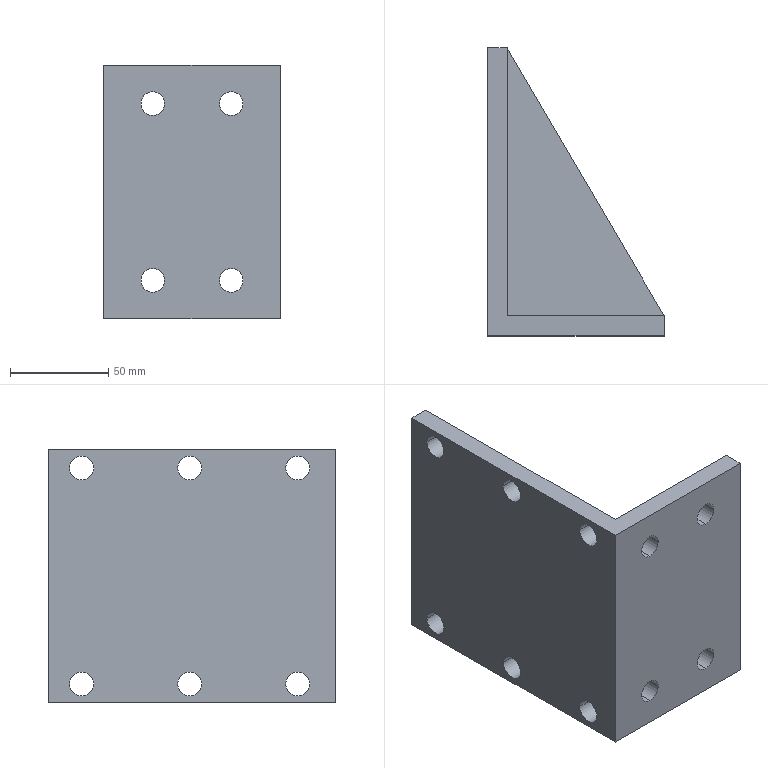Part | SolidWorks | features BaseBody 1, HoleWzd 1 | 1 solid | 33 faces | box 90 x 146.4 x 128.8 mm | volume 334625 mm3 | cylinder 20 | plane 13 | commonest cylinder face diameters 12.2 x12 12 x8
STEP:
#1=CARTESIAN_POINT('',(147.,10.6,14.));
#2=VERTEX_POINT('',#1);
#3=CARTESIAN_POINT('',(147.,10.6,26.));
#4=VERTEX_POINT('',#3);
#5=CARTESIAN_POINT('',(147.,10.6,20.));
#6=DIRECTION('',(0.,1.,0.));
#7=DIRECTION('',(-1.,0.,0.));
#8=AXIS2_PLACEMENT_3D('',#5,#6,#7);
#9=CIRCLE('',#8,6.);
#10=EDGE_CURVE('',#2,#4,#9,.T.);
#11=ORIENTED_EDGE('',*,*,#10,.T.);
#12=CARTESIAN_POINT('',(147.,0.6,26.));
#13=VERTEX_POINT('',#12);
#14=CARTESIAN_POINT('',(147.,0.6,26.));
#15=DIRECTION('',(0.,-1.,0.));
#16=VECTOR('',#15,1000.);
#17=LINE('',#14,#16);
#18=EDGE_CURVE('',#4,#13,#17,.T.);
#19=ORIENTED_EDGE('',*,*,#18,.T.);
#20=CARTESIAN_POINT('',(147.,0.6,14.));
#21=VERTEX_POINT('',#20);
#22=CARTESIAN_POINT('',(147.,0.6,20.));
#23=DIRECTION('',(0.,-1.,0.));
#24=DIRECTION('',(0.,0.,-1.));
#25=AXIS2_PLACEMENT_3D('',#22,#23,#24);
#26=CIRCLE('',#25,6.);
#27=EDGE_CURVE('',#13,#21,#26,.T.);
#28=ORIENTED_EDGE('',*,*,#27,.T.);
#29=CARTESIAN_POINT('',(147.,0.6,14.));
#30=DIRECTION('',(0.,-1.,0.));
#31=VECTOR('',#30,1000.);
#32=LINE('',#29,#31);
#33=EDGE_CURVE('',#2,#21,#32,.T.);
#34=ORIENTED_EDGE('',*,*,#33,.F.);
#35=EDGE_LOOP('',(#11,#19,#28,#34));
#36=FACE_OUTER_BOUND('',#35,.T.);
#37=CARTESIAN_POINT('',(147.,0.6,20.));
#38=DIRECTION('',(0.,-1.,0.));
#39=DIRECTION('',(0.,0.,-1.));
#40=AXIS2_PLACEMENT_3D('',#37,#38,#39);
#41=CYLINDRICAL_SURFACE('',#40,6.);
#42=ADVANCED_FACE('',(#36),#41,.F.);
#43=CARTESIAN_POINT('',(187.,10.6,14.));
#44=VERTEX_POINT('',#43);
#45=CARTESIAN_POINT('',(187.,10.6,26.));
#46=VERTEX_POINT('',#45);
#47=CARTESIAN_POINT('',(187.,10.6,20.));
#48=DIRECTION('',(0.,1.,0.));
#49=DIRECTION('',(-1.,0.,0.));
#50=AXIS2_PLACEMENT_3D('',#47,#48,#49);
#51=CIRCLE('',#50,6.);
#52=EDGE_CURVE('',#44,#46,#51,.T.);
#53=ORIENTED_EDGE('',*,*,#52,.T.);
#54=CARTESIAN_POINT('',(187.,0.6,26.));
#55=VERTEX_POINT('',#54);
#56=CARTESIAN_POINT('',(187.,0.6,26.));
#57=DIRECTION('',(0.,-1.,0.));
#58=VECTOR('',#57,1000.);
#59=LINE('',#56,#58);
#60=EDGE_CURVE('',#46,#55,#59,.T.);
#61=ORIENTED_EDGE('',*,*,#60,.T.);
#62=CARTESIAN_POINT('',(187.,0.6,14.));
#63=VERTEX_POINT('',#62);
#64=CARTESIAN_POINT('',(187.,0.6,20.));
#65=DIRECTION('',(0.,-1.,0.));
#66=DIRECTION('',(0.,0.,-1.));
#67=AXIS2_PLACEMENT_3D('',#64,#65,#66);
#68=CIRCLE('',#67,6.);
#69=EDGE_CURVE('',#55,#63,#68,.T.);
#70=ORIENTED_EDGE('',*,*,#69,.T.);
#71=CARTESIAN_POINT('',(187.,0.6,14.));
#72=DIRECTION('',(0.,-1.,0.));
#73=VECTOR('',#72,1000.);
#74=LINE('',#71,#73);
#75=EDGE_CURVE('',#44,#63,#74,.T.);
#76=ORIENTED_EDGE('',*,*,#75,.F.);
#77=EDGE_LOOP('',(#53,#61,#70,#76));
#78=FACE_OUTER_BOUND('',#77,.T.);
#79=CARTESIAN_POINT('',(187.,0.6,20.));
#80=DIRECTION('',(0.,-1.,0.));
#81=DIRECTION('',(0.,0.,-1.));
#82=AXIS2_PLACEMENT_3D('',#79,#80,#81);
#83=CYLINDRICAL_SURFACE('',#82,6.);
#84=ADVANCED_FACE('',(#78),#83,.F.);
#85=CARTESIAN_POINT('',(187.,10.6,104.));
#86=VERTEX_POINT('',#85);
#87=CARTESIAN_POINT('',(187.,10.6,116.));
#88=VERTEX_POINT('',#87);
#89=CARTESIAN_POINT('',(187.,10.6,110.));
#90=DIRECTION('',(0.,1.,0.));
#91=DIRECTION('',(-1.,0.,0.));
#92=AXIS2_PLACEMENT_3D('',#89,#90,#91);
#93=CIRCLE('',#92,6.);
#94=EDGE_CURVE('',#86,#88,#93,.T.);
#95=ORIENTED_EDGE('',*,*,#94,.T.);
#96=CARTESIAN_POINT('',(187.,0.6,116.));
#97=VERTEX_POINT('',#96);
#98=CARTESIAN_POINT('',(187.,0.6,116.));
#99=DIRECTION('',(0.,-1.,0.));
#100=VECTOR('',#99,1000.);
#101=LINE('',#98,#100);
#102=EDGE_CURVE('',#88,#97,#101,.T.);
#103=ORIENTED_EDGE('',*,*,#102,.T.);
#104=CARTESIAN_POINT('',(187.,0.6,104.));
#105=VERTEX_POINT('',#104);
#106=CARTESIAN_POINT('',(187.,0.6,110.));
#107=DIRECTION('',(0.,-1.,0.));
#108=DIRECTION('',(0.,0.,-1.));
#109=AXIS2_PLACEMENT_3D('',#106,#107,#108);
#110=CIRCLE('',#109,6.);
#111=EDGE_CURVE('',#97,#105,#110,.T.);
#112=ORIENTED_EDGE('',*,*,#111,.T.);
#113=CARTESIAN_POINT('',(187.,0.6,104.));
#114=DIRECTION('',(0.,-1.,0.));
#115=VECTOR('',#114,1000.);
#116=LINE('',#113,#115);
#117=EDGE_CURVE('',#86,#105,#116,.T.);
#118=ORIENTED_EDGE('',*,*,#117,.F.);
#119=EDGE_LOOP('',(#95,#103,#112,#118));
#120=FACE_OUTER_BOUND('',#119,.T.);
#121=CARTESIAN_POINT('',(187.,0.6,110.));
#122=DIRECTION('',(0.,-1.,0.));
#123=DIRECTION('',(0.,0.,-1.));
#124=AXIS2_PLACEMENT_3D('',#121,#122,#123);
#125=CYLINDRICAL_SURFACE('',#124,6.);
#126=ADVANCED_FACE('',(#120),#125,.F.);
#127=CARTESIAN_POINT('',(147.,10.6,104.));
#128=VERTEX_POINT('',#127);
#129=CARTESIAN_POINT('',(147.,10.6,116.));
#130=VERTEX_POINT('',#129);
#131=CARTESIAN_POINT('',(147.,10.6,110.));
#132=DIRECTION('',(0.,1.,0.));
#133=DIRECTION('',(-1.,0.,0.));
#134=AXIS2_PLACEMENT_3D('',#131,#132,#133);
#135=CIRCLE('',#134,6.);
#136=EDGE_CURVE('',#128,#130,#135,.T.);
#137=ORIENTED_EDGE('',*,*,#136,.T.);
#138=CARTESIAN_POINT('',(147.,0.6,116.));
#139=VERTEX_POINT('',#138);
#140=CARTESIAN_POINT('',(147.,0.6,116.));
#141=DIRECTION('',(0.,-1.,0.));
#142=VECTOR('',#141,1000.);
#143=LINE('',#140,#142);
#144=EDGE_CURVE('',#130,#139,#143,.T.);
#145=ORIENTED_EDGE('',*,*,#144,.T.);
#146=CARTESIAN_POINT('',(147.,0.6,104.));
#147=VERTEX_POINT('',#146);
#148=CARTESIAN_POINT('',(147.,0.6,110.));
#149=DIRECTION('',(0.,-1.,0.));
#150=DIRECTION('',(0.,0.,-1.));
#151=AXIS2_PLACEMENT_3D('',#148,#149,#150);
#152=CIRCLE('',#151,6.);
#153=EDGE_CURVE('',#139,#147,#152,.T.);
#154=ORIENTED_EDGE('',*,*,#153,.T.);
#155=CARTESIAN_POINT('',(147.,0.6,104.));
#156=DIRECTION('',(0.,-1.,0.));
#157=VECTOR('',#156,1000.);
#158=LINE('',#155,#157);
#159=EDGE_CURVE('',#128,#147,#158,.T.);
#160=ORIENTED_EDGE('',*,*,#159,.F.);
#161=EDGE_LOOP('',(#137,#145,#154,#160));
#162=FACE_OUTER_BOUND('',#161,.T.);
#163=CARTESIAN_POINT('',(147.,0.6,110.));
#164=DIRECTION('',(0.,-1.,0.));
#165=DIRECTION('',(0.,0.,-1.));
#166=AXIS2_PLACEMENT_3D('',#163,#164,#165);
#167=CYLINDRICAL_SURFACE('',#166,6.);
#168=ADVANCED_FACE('',(#162),#167,.F.);
#169=CARTESIAN_POINT('',(132.,68.9,10.));
#170=VERTEX_POINT('',#169);
#171=CARTESIAN_POINT('',(132.,81.1,10.));
#172=VERTEX_POINT('',#171);
#173=CARTESIAN_POINT('',(132.,75.,10.));
#174=DIRECTION('',(1.,0.,0.));
#175=DIRECTION('',(0.,1.,0.));
#176=AXIS2_PLACEMENT_3D('',#173,#174,#175);
#177=CIRCLE('',#176,6.1);
#178=EDGE_CURVE('',#170,#172,#177,.T.);
#179=ORIENTED_EDGE('',*,*,#178,.T.);
#180=CARTESIAN_POINT('',(122.,81.1,10.));
#181=VERTEX_POINT('',#180);
#182=CARTESIAN_POINT('',(132.,81.1,10.));
#183=DIRECTION('',(-1.,0.,0.));
#184=VECTOR('',#183,1000.);
#185=LINE('',#182,#184);
#186=EDGE_CURVE('',#172,#181,#185,.T.);
#187=ORIENTED_EDGE('',*,*,#186,.T.);
#188=CARTESIAN_POINT('',(122.,68.9,10.));
#189=VERTEX_POINT('',#188);
#190=CARTESIAN_POINT('',(122.,75.,10.));
#191=DIRECTION('',(1.,0.,0.));
#192=DIRECTION('',(0.,1.,0.));
#193=AXIS2_PLACEMENT_3D('',#190,#191,#192);
#194=CIRCLE('',#193,6.1);
#195=EDGE_CURVE('',#189,#181,#194,.T.);
#196=ORIENTED_EDGE('',*,*,#195,.F.);
#197=CARTESIAN_POINT('',(132.,68.9,10.));
#198=DIRECTION('',(-1.,0.,0.));
#199=VECTOR('',#198,1000.);
#200=LINE('',#197,#199);
#201=EDGE_CURVE('',#170,#189,#200,.T.);
#202=ORIENTED_EDGE('',*,*,#201,.F.);
#203=EDGE_LOOP('',(#179,#187,#196,#202));
#204=FACE_OUTER_BOUND('',#203,.T.);
#205=CARTESIAN_POINT('',(132.,75.,10.));
#206=DIRECTION('',(-1.,0.,0.));
#207=DIRECTION('',(0.,-1.,0.));
#208=AXIS2_PLACEMENT_3D('',#205,#206,#207);
#209=CYLINDRICAL_SURFACE('',#208,6.1);
#210=ADVANCED_FACE('',(#204),#209,.F.);
#211=CARTESIAN_POINT('',(132.,123.9,10.));
#212=VERTEX_POINT('',#211);
#213=CARTESIAN_POINT('',(132.,136.1,10.));
#214=VERTEX_POINT('',#213);
#215=CARTESIAN_POINT('',(132.,130.,10.));
#216=DIRECTION('',(1.,0.,0.));
#217=DIRECTION('',(0.,1.,0.));
#218=AXIS2_PLACEMENT_3D('',#215,#216,#217);
#219=CIRCLE('',#218,6.1);
#220=EDGE_CURVE('',#212,#214,#219,.T.);
#221=ORIENTED_EDGE('',*,*,#220,.T.);
#222=CARTESIAN_POINT('',(122.,136.1,10.));
#223=VERTEX_POINT('',#222);
#224=CARTESIAN_POINT('',(132.,136.1,10.));
#225=DIRECTION('',(-1.,0.,0.));
#226=VECTOR('',#225,1000.);
#227=LINE('',#224,#226);
#228=EDGE_CURVE('',#214,#223,#227,.T.);
#229=ORIENTED_EDGE('',*,*,#228,.T.);
#230=CARTESIAN_POINT('',(122.,123.9,10.));
#231=VERTEX_POINT('',#230);
#232=CARTESIAN_POINT('',(122.,130.,10.));
#233=DIRECTION('',(1.,0.,0.));
#234=DIRECTION('',(0.,1.,0.));
#235=AXIS2_PLACEMENT_3D('',#232,#233,#234);
#236=CIRCLE('',#235,6.1);
#237=EDGE_CURVE('',#231,#223,#236,.T.);
#238=ORIENTED_EDGE('',*,*,#237,.F.);
#239=CARTESIAN_POINT('',(132.,123.9,10.));
#240=DIRECTION('',(-1.,0.,0.));
#241=VECTOR('',#240,1000.);
#242=LINE('',#239,#241);
#243=EDGE_CURVE('',#212,#231,#242,.T.);
#244=ORIENTED_EDGE('',*,*,#243,.F.);
#245=EDGE_LOOP('',(#221,#229,#238,#244));
#246=FACE_OUTER_BOUND('',#245,.T.);
#247=CARTESIAN_POINT('',(132.,130.,10.));
#248=DIRECTION('',(-1.,0.,0.));
#249=DIRECTION('',(0.,-1.,0.));
#250=AXIS2_PLACEMENT_3D('',#247,#248,#249);
#251=CYLINDRICAL_SURFACE('',#250,6.1);
#252=ADVANCED_FACE('',(#246),#251,.F.);
#253=CARTESIAN_POINT('',(132.,123.9,120.));
#254=VERTEX_POINT('',#253);
#255=CARTESIAN_POINT('',(132.,136.1,120.));
#256=VERTEX_POINT('',#255);
#257=CARTESIAN_POINT('',(132.,130.,120.));
#258=DIRECTION('',(1.,0.,0.));
#259=DIRECTION('',(0.,1.,0.));
#260=AXIS2_PLACEMENT_3D('',#257,#258,#259);
#261=CIRCLE('',#260,6.1);
#262=EDGE_CURVE('',#254,#256,#261,.T.);
#263=ORIENTED_EDGE('',*,*,#262,.T.);
#264=CARTESIAN_POINT('',(122.,136.1,120.));
#265=VERTEX_POINT('',#264);
#266=CARTESIAN_POINT('',(132.,136.1,120.));
#267=DIRECTION('',(-1.,0.,0.));
#268=VECTOR('',#267,1000.);
#269=LINE('',#266,#268);
#270=EDGE_CURVE('',#256,#265,#269,.T.);
#271=ORIENTED_EDGE('',*,*,#270,.T.);
#272=CARTESIAN_POINT('',(122.,123.9,120.));
#273=VERTEX_POINT('',#272);
#274=CARTESIAN_POINT('',(122.,130.,120.));
#275=DIRECTION('',(1.,0.,0.));
#276=DIRECTION('',(0.,1.,0.));
#277=AXIS2_PLACEMENT_3D('',#274,#275,#276);
#278=CIRCLE('',#277,6.1);
#279=EDGE_CURVE('',#273,#265,#278,.T.);
#280=ORIENTED_EDGE('',*,*,#279,.F.);
#281=CARTESIAN_POINT('',(132.,123.9,120.));
#282=DIRECTION('',(-1.,0.,0.));
#283=VECTOR('',#282,1000.);
#284=LINE('',#281,#283);
#285=EDGE_CURVE('',#254,#273,#284,.T.);
#286=ORIENTED_EDGE('',*,*,#285,.F.);
#287=EDGE_LOOP('',(#263,#271,#280,#286));
#288=FACE_OUTER_BOUND('',#287,.T.);
#289=CARTESIAN_POINT('',(132.,130.,120.));
#290=DIRECTION('',(-1.,0.,0.));
#291=DIRECTION('',(0.,-1.,0.));
#292=AXIS2_PLACEMENT_3D('',#289,#290,#291);
#293=CYLINDRICAL_SURFACE('',#292,6.1);
#294=ADVANCED_FACE('',(#288),#293,.F.);
#295=CARTESIAN_POINT('',(132.,68.9,120.));
#296=VERTEX_POINT('',#295);
#297=CARTESIAN_POINT('',(132.,81.1,120.));
#298=VERTEX_POINT('',#297);
#299=CARTESIAN_POINT('',(132.,75.,120.));
#300=DIRECTION('',(1.,0.,0.));
#301=DIRECTION('',(0.,1.,0.));
#302=AXIS2_PLACEMENT_3D('',#299,#300,#301);
#303=CIRCLE('',#302,6.1);
#304=EDGE_CURVE('',#296,#298,#303,.T.);
#305=ORIENTED_EDGE('',*,*,#304,.T.);
#306=CARTESIAN_POINT('',(122.,81.1,120.));
#307=VERTEX_POINT('',#306);
#308=CARTESIAN_POINT('',(132.,81.1,120.));
#309=DIRECTION('',(-1.,0.,0.));
#310=VECTOR('',#309,1000.);
#311=LINE('',#308,#310);
#312=EDGE_CURVE('',#298,#307,#311,.T.);
#313=ORIENTED_EDGE('',*,*,#312,.T.);
#314=CARTESIAN_POINT('',(122.,68.9,120.));
#315=VERTEX_POINT('',#314);
#316=CARTESIAN_POINT('',(122.,75.,120.));
#317=DIRECTION('',(1.,0.,0.));
#318=DIRECTION('',(0.,1.,0.));
#319=AXIS2_PLACEMENT_3D('',#316,#317,#318);
#320=CIRCLE('',#319,6.1);
#321=EDGE_CURVE('',#315,#307,#320,.T.);
#322=ORIENTED_EDGE('',*,*,#321,.F.);
#323=CARTESIAN_POINT('',(132.,68.9,120.));
#324=DIRECTION('',(-1.,0.,0.));
#325=VECTOR('',#324,1000.);
#326=LINE('',#323,#325);
#327=EDGE_CURVE('',#296,#315,#326,.T.);
#328=ORIENTED_EDGE('',*,*,#327,.F.);
#329=EDGE_LOOP('',(#305,#313,#322,#328));
#330=FACE_OUTER_BOUND('',#329,.T.);
#331=CARTESIAN_POINT('',(132.,75.,120.));
#332=DIRECTION('',(-1.,0.,0.));
#333=DIRECTION('',(0.,-1.,0.));
#334=AXIS2_PLACEMENT_3D('',#331,#332,#333);
#335=CYLINDRICAL_SURFACE('',#334,6.1);
#336=ADVANCED_FACE('',(#330),#335,.F.);
#337=CARTESIAN_POINT('',(132.,13.9,120.));
#338=VERTEX_POINT('',#337);
#339=CARTESIAN_POINT('',(132.,26.1,120.));
#340=VERTEX_POINT('',#339);
#341=CARTESIAN_POINT('',(132.,20.,120.));
#342=DIRECTION('',(1.,0.,0.));
#343=DIRECTION('',(0.,1.,0.));
#344=AXIS2_PLACEMENT_3D('',#341,#342,#343);
#345=CIRCLE('',#344,6.1);
#346=EDGE_CURVE('',#338,#340,#345,.T.);
#347=ORIENTED_EDGE('',*,*,#346,.T.);
#348=CARTESIAN_POINT('',(122.,26.1,120.));
#349=VERTEX_POINT('',#348);
#350=CARTESIAN_POINT('',(132.,26.1,120.));
#351=DIRECTION('',(-1.,0.,0.));
#352=VECTOR('',#351,1000.);
#353=LINE('',#350,#352);
#354=EDGE_CURVE('',#340,#349,#353,.T.);
#355=ORIENTED_EDGE('',*,*,#354,.T.);
#356=CARTESIAN_POINT('',(122.,13.9,120.));
#357=VERTEX_POINT('',#356);
#358=CARTESIAN_POINT('',(122.,20.,120.));
#359=DIRECTION('',(1.,0.,0.));
#360=DIRECTION('',(0.,1.,0.));
#361=AXIS2_PLACEMENT_3D('',#358,#359,#360);
#362=CIRCLE('',#361,6.1);
#363=EDGE_CURVE('',#357,#349,#362,.T.);
#364=ORIENTED_EDGE('',*,*,#363,.F.);
#365=CARTESIAN_POINT('',(132.,13.9,120.));
#366=DIRECTION('',(-1.,0.,0.));
#367=VECTOR('',#366,1000.);
#368=LINE('',#365,#367);
#369=EDGE_CURVE('',#338,#357,#368,.T.);
#370=ORIENTED_EDGE('',*,*,#369,.F.);
#371=EDGE_LOOP('',(#347,#355,#364,#370));
#372=FACE_OUTER_BOUND('',#371,.T.);
#373=CARTESIAN_POINT('',(132.,20.,120.));
#374=DIRECTION('',(-1.,0.,0.));
#375=DIRECTION('',(0.,-1.,0.));
#376=AXIS2_PLACEMENT_3D('',#373,#374,#375);
#377=CYLINDRICAL_SURFACE('',#376,6.1);
#378=ADVANCED_FACE('',(#372),#377,.F.);
#379=CARTESIAN_POINT('',(132.,13.9,10.));
#380=VERTEX_POINT('',#379);
#381=CARTESIAN_POINT('',(132.,26.1,10.));
#382=VERTEX_POINT('',#381);
#383=CARTESIAN_POINT('',(132.,20.,10.));
#384=DIRECTION('',(1.,0.,0.));
#385=DIRECTION('',(0.,1.,0.));
#386=AXIS2_PLACEMENT_3D('',#383,#384,#385);
#387=CIRCLE('',#386,6.1);
#388=EDGE_CURVE('',#380,#382,#387,.T.);
#389=ORIENTED_EDGE('',*,*,#388,.T.);
#390=CARTESIAN_POINT('',(122.,26.1,10.));
#391=VERTEX_POINT('',#390);
#392=CARTESIAN_POINT('',(132.,26.1,10.));
#393=DIRECTION('',(-1.,0.,0.));
#394=VECTOR('',#393,1000.);
#395=LINE('',#392,#394);
#396=EDGE_CURVE('',#382,#391,#395,.T.);
#397=ORIENTED_EDGE('',*,*,#396,.T.);
#398=CARTESIAN_POINT('',(122.,13.9,10.));
#399=VERTEX_POINT('',#398);
#400=CARTESIAN_POINT('',(122.,20.,10.));
#401=DIRECTION('',(1.,0.,0.));
#402=DIRECTION('',(0.,1.,0.));
#403=AXIS2_PLACEMENT_3D('',#400,#401,#402);
#404=CIRCLE('',#403,6.1);
#405=EDGE_CURVE('',#399,#391,#404,.T.);
#406=ORIENTED_EDGE('',*,*,#405,.F.);
#407=CARTESIAN_POINT('',(132.,13.9,10.));
#408=DIRECTION('',(-1.,0.,0.));
#409=VECTOR('',#408,1000.);
#410=LINE('',#407,#409);
#411=EDGE_CURVE('',#380,#399,#410,.T.);
#412=ORIENTED_EDGE('',*,*,#411,.F.);
#413=EDGE_LOOP('',(#389,#397,#406,#412));
#414=FACE_OUTER_BOUND('',#413,.T.);
#415=CARTESIAN_POINT('',(132.,20.,10.));
#416=DIRECTION('',(-1.,0.,0.));
#417=DIRECTION('',(0.,-1.,0.));
#418=AXIS2_PLACEMENT_3D('',#415,#416,#417);
#419=CYLINDRICAL_SURFACE('',#418,6.1);
#420=ADVANCED_FACE('',(#414),#419,.F.);
#421=ORIENTED_EDGE('',*,*,#262,.F.);
#422=CARTESIAN_POINT('',(132.,130.,120.));
#423=DIRECTION('',(1.,0.,0.));
#424=DIRECTION('',(0.,1.,0.));
#425=AXIS2_PLACEMENT_3D('',#422,#423,#424);
#426=CIRCLE('',#425,6.1);
#427=EDGE_CURVE('',#256,#254,#426,.T.);
#428=ORIENTED_EDGE('',*,*,#427,.F.);
#429=EDGE_LOOP('',(#421,#428));
#430=FACE_BOUND('',#429,.T.);
#431=ORIENTED_EDGE('',*,*,#346,.F.);
#432=CARTESIAN_POINT('',(132.,20.,120.));
#433=DIRECTION('',(1.,0.,0.));
#434=DIRECTION('',(0.,1.,0.));
#435=AXIS2_PLACEMENT_3D('',#432,#433,#434);
#436=CIRCLE('',#435,6.1);
#437=EDGE_CURVE('',#340,#338,#436,.T.);
#438=ORIENTED_EDGE('',*,*,#437,.F.);
#439=EDGE_LOOP('',(#431,#438));
#440=FACE_BOUND('',#439,.T.);
#441=ORIENTED_EDGE('',*,*,#304,.F.);
#442=CARTESIAN_POINT('',(132.,75.,120.));
#443=DIRECTION('',(1.,0.,0.));
#444=DIRECTION('',(0.,1.,0.));
#445=AXIS2_PLACEMENT_3D('',#442,#443,#444);
#446=CIRCLE('',#445,6.1);
#447=EDGE_CURVE('',#298,#296,#446,.T.);
#448=ORIENTED_EDGE('',*,*,#447,.F.);
#449=EDGE_LOOP('',(#441,#448));
#450=FACE_BOUND('',#449,.T.);
#451=CARTESIAN_POINT('',(132.,10.6,129.4));
#452=VERTEX_POINT('',#451);
#453=CARTESIAN_POINT('',(132.,10.6,70.));
#454=VERTEX_POINT('',#453);
#455=CARTESIAN_POINT('',(132.,10.6,129.4));
#456=DIRECTION('',(0.,0.,-1.));
#457=VECTOR('',#456,1000.);
#458=LINE('',#455,#457);
#459=EDGE_CURVE('',#452,#454,#458,.T.);
#460=ORIENTED_EDGE('',*,*,#459,.T.);
#461=CARTESIAN_POINT('',(132.,147.,70.));
#462=VERTEX_POINT('',#461);
#463=CARTESIAN_POINT('',(132.,10.6,70.));
#464=DIRECTION('',(0.,1.,0.));
#465=VECTOR('',#464,1000.);
#466=LINE('',#463,#465);
#467=EDGE_CURVE('',#454,#462,#466,.T.);
#468=ORIENTED_EDGE('',*,*,#467,.T.);
#469=CARTESIAN_POINT('',(132.,147.,129.4));
#470=VERTEX_POINT('',#469);
#471=CARTESIAN_POINT('',(132.,147.,0.6));
#472=DIRECTION('',(0.,0.,1.));
#473=VECTOR('',#472,1000.);
#474=LINE('',#471,#473);
#475=EDGE_CURVE('',#462,#470,#474,.T.);
#476=ORIENTED_EDGE('',*,*,#475,.T.);
#477=CARTESIAN_POINT('',(132.,147.,129.4));
#478=DIRECTION('',(0.,-1.,0.));
#479=VECTOR('',#478,1000.);
#480=LINE('',#477,#479);
#481=EDGE_CURVE('',#470,#452,#480,.T.);
#482=ORIENTED_EDGE('',*,*,#481,.T.);
#483=EDGE_LOOP('',(#460,#468,#476,#482));
#484=FACE_OUTER_BOUND('',#483,.T.);
#485=CARTESIAN_POINT('',(132.,0.,0.));
#486=DIRECTION('',(1.,0.,0.));
#487=DIRECTION('',(0.,1.,0.));
#488=AXIS2_PLACEMENT_3D('',#485,#486,#487);
#489=PLANE('',#488);
#490=ADVANCED_FACE('',(#430,#440,#450,#484),#489,.T.);
#491=ORIENTED_EDGE('',*,*,#94,.F.);
#492=CARTESIAN_POINT('',(187.,10.6,110.));
#493=DIRECTION('',(0.,1.,0.));
#494=DIRECTION('',(-1.,0.,0.));
#495=AXIS2_PLACEMENT_3D('',#492,#493,#494);
#496=CIRCLE('',#495,6.);
#497=EDGE_CURVE('',#88,#86,#496,.T.);
#498=ORIENTED_EDGE('',*,*,#497,.F.);
#499=EDGE_LOOP('',(#491,#498));
#500=FACE_BOUND('',#499,.T.);
#501=ORIENTED_EDGE('',*,*,#136,.F.);
#502=CARTESIAN_POINT('',(147.,10.6,110.));
#503=DIRECTION('',(0.,1.,0.));
#504=DIRECTION('',(-1.,0.,0.));
#505=AXIS2_PLACEMENT_3D('',#502,#503,#504);
#506=CIRCLE('',#505,6.);
#507=EDGE_CURVE('',#130,#128,#506,.T.);
#508=ORIENTED_EDGE('',*,*,#507,.F.);
#509=EDGE_LOOP('',(#501,#508));
#510=FACE_BOUND('',#509,.T.);
#511=CARTESIAN_POINT('',(212.,10.6,129.4));
#512=VERTEX_POINT('',#511);
#513=CARTESIAN_POINT('',(212.,10.6,70.));
#514=VERTEX_POINT('',#513);
#515=CARTESIAN_POINT('',(212.,10.6,129.4));
#516=DIRECTION('',(0.,0.,-1.));
#517=VECTOR('',#516,1000.);
#518=LINE('',#515,#517);
#519=EDGE_CURVE('',#512,#514,#518,.T.);
#520=ORIENTED_EDGE('',*,*,#519,.T.);
#521=CARTESIAN_POINT('',(212.,10.6,70.));
#522=DIRECTION('',(-1.,0.,0.));
#523=VECTOR('',#522,1000.);
#524=LINE('',#521,#523);
#525=EDGE_CURVE('',#514,#454,#524,.T.);
#526=ORIENTED_EDGE('',*,*,#525,.T.);
#527=ORIENTED_EDGE('',*,*,#459,.F.);
#528=CARTESIAN_POINT('',(212.,10.6,129.4));
#529=DIRECTION('',(-1.,0.,0.));
#530=VECTOR('',#529,1000.);
#531=LINE('',#528,#530);
#532=EDGE_CURVE('',#512,#452,#531,.T.);
#533=ORIENTED_EDGE('',*,*,#532,.F.);
#534=EDGE_LOOP('',(#520,#526,#527,#533));
#535=FACE_OUTER_BOUND('',#534,.T.);
#536=CARTESIAN_POINT('',(212.,10.6,129.4));
#537=DIRECTION('',(0.,1.,0.));
#538=DIRECTION('',(-1.,0.,0.));
#539=AXIS2_PLACEMENT_3D('',#536,#537,#538);
#540=PLANE('',#539);
#541=ADVANCED_FACE('',(#500,#510,#535),#540,.T.);
#542=CARTESIAN_POINT('',(132.,10.6,60.));
#543=VERTEX_POINT('',#542);
#544=CARTESIAN_POINT('',(132.,147.,60.));
#545=VERTEX_POINT('',#544);
#546=CARTESIAN_POINT('',(132.,10.6,60.));
#547=DIRECTION('',(0.,1.,0.));
#548=VECTOR('',#547,1000.);
#549=LINE('',#546,#548);
#550=EDGE_CURVE('',#543,#545,#549,.T.);
#551=ORIENTED_EDGE('',*,*,#550,.F.);
#552=CARTESIAN_POINT('',(132.,10.6,0.6));
#553=VERTEX_POINT('',#552);
#554=CARTESIAN_POINT('',(132.,10.6,129.4));
#555=DIRECTION('',(0.,0.,-1.));
#556=VECTOR('',#555,1000.);
#557=LINE('',#554,#556);
#558=EDGE_CURVE('',#543,#553,#557,.T.);
#559=ORIENTED_EDGE('',*,*,#558,.T.);
#560=CARTESIAN_POINT('',(132.,147.,0.6));
#561=VERTEX_POINT('',#560);
#562=CARTESIAN_POINT('',(132.,0.6,0.6));
#563=DIRECTION('',(0.,1.,0.));
#564=VECTOR('',#563,1000.);
#565=LINE('',#562,#564);
#566=EDGE_CURVE('',#553,#561,#565,.T.);
#567=ORIENTED_EDGE('',*,*,#566,.T.);
#568=CARTESIAN_POINT('',(132.,147.,0.6));
#569=DIRECTION('',(0.,0.,1.));
#570=VECTOR('',#569,1000.);
#571=LINE('',#568,#570);
#572=EDGE_CURVE('',#561,#545,#571,.T.);
#573=ORIENTED_EDGE('',*,*,#572,.T.);
#574=EDGE_LOOP('',(#551,#559,#567,#573));
#575=FACE_OUTER_BOUND('',#574,.T.);
#576=ORIENTED_EDGE('',*,*,#220,.F.);
#577=CARTESIAN_POINT('',(132.,130.,10.));
#578=DIRECTION('',(1.,0.,0.));
#579=DIRECTION('',(0.,1.,0.));
#580=AXIS2_PLACEMENT_3D('',#577,#578,#579);
#581=CIRCLE('',#580,6.1);
#582=EDGE_CURVE('',#214,#212,#581,.T.);
#583=ORIENTED_EDGE('',*,*,#582,.F.);
#584=EDGE_LOOP('',(#576,#583));
#585=FACE_BOUND('',#584,.T.);
#586=ORIENTED_EDGE('',*,*,#388,.F.);
#587=CARTESIAN_POINT('',(132.,20.,10.));
#588=DIRECTION('',(1.,0.,0.));
#589=DIRECTION('',(0.,1.,0.));
#590=AXIS2_PLACEMENT_3D('',#587,#588,#589);
#591=CIRCLE('',#590,6.1);
#592=EDGE_CURVE('',#382,#380,#591,.T.);
#593=ORIENTED_EDGE('',*,*,#592,.F.);
#594=EDGE_LOOP('',(#586,#593));
#595=FACE_BOUND('',#594,.T.);
#596=ORIENTED_EDGE('',*,*,#178,.F.);
#597=CARTESIAN_POINT('',(132.,75.,10.));
#598=DIRECTION('',(1.,0.,0.));
#599=DIRECTION('',(0.,1.,0.));
#600=AXIS2_PLACEMENT_3D('',#597,#598,#599);
#601=CIRCLE('',#600,6.1);
#602=EDGE_CURVE('',#172,#170,#601,.T.);
#603=ORIENTED_EDGE('',*,*,#602,.F.);
#604=EDGE_LOOP('',(#596,#603));
#605=FACE_BOUND('',#604,.T.);
#606=CARTESIAN_POINT('',(132.,0.,0.));
#607=DIRECTION('',(1.,0.,0.));
#608=DIRECTION('',(0.,1.,0.));
#609=AXIS2_PLACEMENT_3D('',#606,#607,#608);
#610=PLANE('',#609);
#611=ADVANCED_FACE('',(#575,#585,#595,#605),#610,.T.);
#612=CARTESIAN_POINT('',(122.,0.6,129.4));
#613=VERTEX_POINT('',#612);
#614=CARTESIAN_POINT('',(122.,0.6,0.6));
#615=VERTEX_POINT('',#614);
#616=CARTESIAN_POINT('',(122.,0.6,129.4));
#617=DIRECTION('',(0.,0.,-1.));
#618=VECTOR('',#617,1000.);
#619=LINE('',#616,#618);
#620=EDGE_CURVE('',#613,#615,#619,.T.);
#621=ORIENTED_EDGE('',*,*,#620,.F.);
#622=CARTESIAN_POINT('',(122.,147.,129.4));
#623=VERTEX_POINT('',#622);
#624=CARTESIAN_POINT('',(122.,147.,129.4));
#625=DIRECTION('',(0.,-1.,0.));
#626=VECTOR('',#625,1000.);
#627=LINE('',#624,#626);
#628=EDGE_CURVE('',#623,#613,#627,.T.);
#629=ORIENTED_EDGE('',*,*,#628,.F.);
#630=CARTESIAN_POINT('',(122.,147.,0.6));
#631=VERTEX_POINT('',#630);
#632=CARTESIAN_POINT('',(122.,147.,0.6));
#633=DIRECTION('',(0.,0.,1.));
#634=VECTOR('',#633,1000.);
#635=LINE('',#632,#634);
#636=EDGE_CURVE('',#631,#623,#635,.T.);
#637=ORIENTED_EDGE('',*,*,#636,.F.);
#638=CARTESIAN_POINT('',(122.,0.6,0.6));
#639=DIRECTION('',(0.,1.,0.));
#640=VECTOR('',#639,1000.);
#641=LINE('',#638,#640);
#642=EDGE_CURVE('',#615,#631,#641,.T.);
#643=ORIENTED_EDGE('',*,*,#642,.F.);
#644=EDGE_LOOP('',(#621,#629,#637,#643));
#645=FACE_OUTER_BOUND('',#644,.T.);
#646=ORIENTED_EDGE('',*,*,#405,.T.);
#647=CARTESIAN_POINT('',(122.,20.,10.));
#648=DIRECTION('',(1.,0.,0.));
#649=DIRECTION('',(0.,1.,0.));
#650=AXIS2_PLACEMENT_3D('',#647,#648,#649);
#651=CIRCLE('',#650,6.1);
#652=EDGE_CURVE('',#391,#399,#651,.T.);
#653=ORIENTED_EDGE('',*,*,#652,.T.);
#654=EDGE_LOOP('',(#646,#653));
#655=FACE_BOUND('',#654,.T.);
#656=ORIENTED_EDGE('',*,*,#363,.T.);
#657=CARTESIAN_POINT('',(122.,20.,120.));
#658=DIRECTION('',(1.,0.,0.));
#659=DIRECTION('',(0.,1.,0.));
#660=AXIS2_PLACEMENT_3D('',#657,#658,#659);
#661=CIRCLE('',#660,6.1);
#662=EDGE_CURVE('',#349,#357,#661,.T.);
#663=ORIENTED_EDGE('',*,*,#662,.T.);
#664=EDGE_LOOP('',(#656,#663));
#665=FACE_BOUND('',#664,.T.);
#666=ORIENTED_EDGE('',*,*,#321,.T.);
#667=CARTESIAN_POINT('',(122.,75.,120.));
#668=DIRECTION('',(1.,0.,0.));
#669=DIRECTION('',(0.,1.,0.));
#670=AXIS2_PLACEMENT_3D('',#667,#668,#669);
#671=CIRCLE('',#670,6.1);
#672=EDGE_CURVE('',#307,#315,#671,.T.);
#673=ORIENTED_EDGE('',*,*,#672,.T.);
#674=EDGE_LOOP('',(#666,#673));
#675=FACE_BOUND('',#674,.T.);
#676=ORIENTED_EDGE('',*,*,#279,.T.);
#677=CARTESIAN_POINT('',(122.,130.,120.));
#678=DIRECTION('',(1.,0.,0.));
#679=DIRECTION('',(0.,1.,0.));
#680=AXIS2_PLACEMENT_3D('',#677,#678,#679);
#681=CIRCLE('',#680,6.1);
#682=EDGE_CURVE('',#265,#273,#681,.T.);
#683=ORIENTED_EDGE('',*,*,#682,.T.);
#684=EDGE_LOOP('',(#676,#683));
#685=FACE_BOUND('',#684,.T.);
#686=ORIENTED_EDGE('',*,*,#237,.T.);
#687=CARTESIAN_POINT('',(122.,130.,10.));
#688=DIRECTION('',(1.,0.,0.));
#689=DIRECTION('',(0.,1.,0.));
#690=AXIS2_PLACEMENT_3D('',#687,#688,#689);
#691=CIRCLE('',#690,6.1);
#692=EDGE_CURVE('',#223,#231,#691,.T.);
#693=ORIENTED_EDGE('',*,*,#692,.T.);
#694=EDGE_LOOP('',(#686,#693));
#695=FACE_BOUND('',#694,.T.);
#696=ORIENTED_EDGE('',*,*,#195,.T.);
#697=CARTESIAN_POINT('',(122.,75.,10.));
#698=DIRECTION('',(1.,0.,0.));
#699=DIRECTION('',(0.,1.,0.));
#700=AXIS2_PLACEMENT_3D('',#697,#698,#699);
#701=CIRCLE('',#700,6.1);
#702=EDGE_CURVE('',#181,#189,#701,.T.);
#703=ORIENTED_EDGE('',*,*,#702,.T.);
#704=EDGE_LOOP('',(#696,#703));
#705=FACE_BOUND('',#704,.T.);
#706=CARTESIAN_POINT('',(122.,0.,0.));
#707=DIRECTION('',(1.,0.,0.));
#708=DIRECTION('',(0.,1.,0.));
#709=AXIS2_PLACEMENT_3D('',#706,#707,#708);
#710=PLANE('',#709);
#711=ADVANCED_FACE('',(#645,#655,#665,#675,#685,#695,#705),#710,.F.);
#712=CARTESIAN_POINT('',(147.,0.6,20.));
#713=DIRECTION('',(0.,-1.,0.));
#714=DIRECTION('',(0.,0.,-1.));
#715=AXIS2_PLACEMENT_3D('',#712,#713,#714);
#716=CIRCLE('',#715,6.);
#717=EDGE_CURVE('',#21,#13,#716,.T.);
#718=ORIENTED_EDGE('',*,*,#717,.F.);
#719=ORIENTED_EDGE('',*,*,#27,.F.);
#720=EDGE_LOOP('',(#718,#719));
#721=FACE_BOUND('',#720,.T.);
#722=CARTESIAN_POINT('',(187.,0.6,20.));
#723=DIRECTION('',(0.,-1.,0.));
#724=DIRECTION('',(0.,0.,-1.));
#725=AXIS2_PLACEMENT_3D('',#722,#723,#724);
#726=CIRCLE('',#725,6.);
#727=EDGE_CURVE('',#63,#55,#726,.T.);
#728=ORIENTED_EDGE('',*,*,#727,.F.);
#729=ORIENTED_EDGE('',*,*,#69,.F.);
#730=EDGE_LOOP('',(#728,#729));
#731=FACE_BOUND('',#730,.T.);
#732=CARTESIAN_POINT('',(187.,0.6,110.));
#733=DIRECTION('',(0.,-1.,0.));
#734=DIRECTION('',(0.,0.,-1.));
#735=AXIS2_PLACEMENT_3D('',#732,#733,#734);
#736=CIRCLE('',#735,6.);
#737=EDGE_CURVE('',#105,#97,#736,.T.);
#738=ORIENTED_EDGE('',*,*,#737,.F.);
#739=ORIENTED_EDGE('',*,*,#111,.F.);
#740=EDGE_LOOP('',(#738,#739));
#741=FACE_BOUND('',#740,.T.);
#742=CARTESIAN_POINT('',(147.,0.6,110.));
#743=DIRECTION('',(0.,-1.,0.));
#744=DIRECTION('',(0.,0.,-1.));
#745=AXIS2_PLACEMENT_3D('',#742,#743,#744);
#746=CIRCLE('',#745,6.);
#747=EDGE_CURVE('',#147,#139,#746,.T.);
#748=ORIENTED_EDGE('',*,*,#747,.F.);
#749=ORIENTED_EDGE('',*,*,#153,.F.);
#750=EDGE_LOOP('',(#748,#749));
#751=FACE_BOUND('',#750,.T.);
#752=ORIENTED_EDGE('',*,*,#620,.T.);
#753=CARTESIAN_POINT('',(212.,0.6,0.6));
#754=VERTEX_POINT('',#753);
#755=CARTESIAN_POINT('',(132.,0.6,0.6));
#756=DIRECTION('',(-1.,0.,0.));
#757=VECTOR('',#756,1000.);
#758=LINE('',#755,#757);
#759=EDGE_CURVE('',#754,#615,#758,.T.);
#760=ORIENTED_EDGE('',*,*,#759,.F.);
#761=CARTESIAN_POINT('',(212.,0.6,129.4));
#762=VERTEX_POINT('',#761);
#763=CARTESIAN_POINT('',(212.,0.6,129.4));
#764=DIRECTION('',(0.,0.,-1.));
#765=VECTOR('',#764,1000.);
#766=LINE('',#763,#765);
#767=EDGE_CURVE('',#762,#754,#766,.T.);
#768=ORIENTED_EDGE('',*,*,#767,.F.);
#769=CARTESIAN_POINT('',(132.,0.6,129.4));
#770=DIRECTION('',(-1.,0.,0.));
#771=VECTOR('',#770,1000.);
#772=LINE('',#769,#771);
#773=EDGE_CURVE('',#762,#613,#772,.T.);
#774=ORIENTED_EDGE('',*,*,#773,.T.);
#775=EDGE_LOOP('',(#752,#760,#768,#774));
#776=FACE_OUTER_BOUND('',#775,.T.);
#777=CARTESIAN_POINT('',(132.,0.6,129.4));
#778=DIRECTION('',(0.,1.,0.));
#779=DIRECTION('',(-1.,0.,0.));
#780=AXIS2_PLACEMENT_3D('',#777,#778,#779);
#781=PLANE('',#780);
#782=ADVANCED_FACE('',(#721,#731,#741,#751,#776),#781,.F.);
#783=ORIENTED_EDGE('',*,*,#642,.T.);
#784=CARTESIAN_POINT('',(132.,147.,0.6));
#785=DIRECTION('',(-1.,0.,0.));
#786=VECTOR('',#785,1000.);
#787=LINE('',#784,#786);
#788=EDGE_CURVE('',#561,#631,#787,.T.);
#789=ORIENTED_EDGE('',*,*,#788,.F.);
#790=ORIENTED_EDGE('',*,*,#566,.F.);
#791=CARTESIAN_POINT('',(212.,10.6,0.6));
#792=VERTEX_POINT('',#791);
#793=CARTESIAN_POINT('',(212.,10.6,0.6));
#794=DIRECTION('',(-1.,0.,0.));
#795=VECTOR('',#794,1000.);
#796=LINE('',#793,#795);
#797=EDGE_CURVE('',#792,#553,#796,.T.);
#798=ORIENTED_EDGE('',*,*,#797,.F.);
#799=CARTESIAN_POINT('',(212.,10.6,0.6));
#800=DIRECTION('',(0.,-1.,0.));
#801=VECTOR('',#800,1000.);
#802=LINE('',#799,#801);
#803=EDGE_CURVE('',#792,#754,#802,.T.);
#804=ORIENTED_EDGE('',*,*,#803,.T.);
#805=ORIENTED_EDGE('',*,*,#759,.T.);
#806=EDGE_LOOP('',(#783,#789,#790,#798,#804,#805));
#807=FACE_OUTER_BOUND('',#806,.T.);
#808=CARTESIAN_POINT('',(132.,0.6,0.6));
#809=DIRECTION('',(0.,0.,1.));
#810=DIRECTION('',(0.,-1.,0.));
#811=AXIS2_PLACEMENT_3D('',#808,#809,#810);
#812=PLANE('',#811);
#813=ADVANCED_FACE('',(#807),#812,.F.);
#814=ORIENTED_EDGE('',*,*,#636,.T.);
#815=CARTESIAN_POINT('',(132.,147.,129.4));
#816=DIRECTION('',(-1.,0.,0.));
#817=VECTOR('',#816,1000.);
#818=LINE('',#815,#817);
#819=EDGE_CURVE('',#470,#623,#818,.T.);
#820=ORIENTED_EDGE('',*,*,#819,.F.);
#821=ORIENTED_EDGE('',*,*,#475,.F.);
#822=CARTESIAN_POINT('',(132.,147.,60.));
#823=DIRECTION('',(0.,0.,1.));
#824=VECTOR('',#823,1000.);
#825=LINE('',#822,#824);
#826=EDGE_CURVE('',#545,#462,#825,.T.);
#827=ORIENTED_EDGE('',*,*,#826,.F.);
#828=ORIENTED_EDGE('',*,*,#572,.F.);
#829=ORIENTED_EDGE('',*,*,#788,.T.);
#830=EDGE_LOOP('',(#814,#820,#821,#827,#828,#829));
#831=FACE_OUTER_BOUND('',#830,.T.);
#832=CARTESIAN_POINT('',(132.,147.,0.6));
#833=DIRECTION('',(0.,-1.,0.));
#834=DIRECTION('',(0.,0.,-1.));
#835=AXIS2_PLACEMENT_3D('',#832,#833,#834);
#836=PLANE('',#835);
#837=ADVANCED_FACE('',(#831),#836,.F.);
#838=ORIENTED_EDGE('',*,*,#628,.T.);
#839=ORIENTED_EDGE('',*,*,#773,.F.);
#840=CARTESIAN_POINT('',(212.,0.6,129.4));
#841=DIRECTION('',(0.,1.,0.));
#842=VECTOR('',#841,1000.);
#843=LINE('',#840,#842);
#844=EDGE_CURVE('',#762,#512,#843,.T.);
#845=ORIENTED_EDGE('',*,*,#844,.T.);
#846=ORIENTED_EDGE('',*,*,#532,.T.);
#847=ORIENTED_EDGE('',*,*,#481,.F.);
#848=ORIENTED_EDGE('',*,*,#819,.T.);
#849=EDGE_LOOP('',(#838,#839,#845,#846,#847,#848));
#850=FACE_OUTER_BOUND('',#849,.T.);
#851=CARTESIAN_POINT('',(132.,147.,129.4));
#852=DIRECTION('',(0.,0.,-1.));
#853=DIRECTION('',(0.,1.,0.));
#854=AXIS2_PLACEMENT_3D('',#851,#852,#853);
#855=PLANE('',#854);
#856=ADVANCED_FACE('',(#850),#855,.F.);
#857=ORIENTED_EDGE('',*,*,#396,.F.);
#858=ORIENTED_EDGE('',*,*,#592,.T.);
#859=ORIENTED_EDGE('',*,*,#411,.T.);
#860=ORIENTED_EDGE('',*,*,#652,.F.);
#861=EDGE_LOOP('',(#857,#858,#859,#860));
#862=FACE_OUTER_BOUND('',#861,.T.);
#863=CARTESIAN_POINT('',(132.,20.,10.));
#864=DIRECTION('',(-1.,0.,0.));
#865=DIRECTION('',(0.,-1.,0.));
#866=AXIS2_PLACEMENT_3D('',#863,#864,#865);
#867=CYLINDRICAL_SURFACE('',#866,6.1);
#868=ADVANCED_FACE('',(#862),#867,.F.);
#869=ORIENTED_EDGE('',*,*,#354,.F.);
#870=ORIENTED_EDGE('',*,*,#437,.T.);
#871=ORIENTED_EDGE('',*,*,#369,.T.);
#872=ORIENTED_EDGE('',*,*,#662,.F.);
#873=EDGE_LOOP('',(#869,#870,#871,#872));
#874=FACE_OUTER_BOUND('',#873,.T.);
#875=CARTESIAN_POINT('',(132.,20.,120.));
#876=DIRECTION('',(-1.,0.,0.));
#877=DIRECTION('',(0.,-1.,0.));
#878=AXIS2_PLACEMENT_3D('',#875,#876,#877);
#879=CYLINDRICAL_SURFACE('',#878,6.1);
#880=ADVANCED_FACE('',(#874),#879,.F.);
#881=ORIENTED_EDGE('',*,*,#312,.F.);
#882=ORIENTED_EDGE('',*,*,#447,.T.);
#883=ORIENTED_EDGE('',*,*,#327,.T.);
#884=ORIENTED_EDGE('',*,*,#672,.F.);
#885=EDGE_LOOP('',(#881,#882,#883,#884));
#886=FACE_OUTER_BOUND('',#885,.T.);
#887=CARTESIAN_POINT('',(132.,75.,120.));
#888=DIRECTION('',(-1.,0.,0.));
#889=DIRECTION('',(0.,-1.,0.));
#890=AXIS2_PLACEMENT_3D('',#887,#888,#889);
#891=CYLINDRICAL_SURFACE('',#890,6.1);
#892=ADVANCED_FACE('',(#886),#891,.F.);
#893=ORIENTED_EDGE('',*,*,#270,.F.);
#894=ORIENTED_EDGE('',*,*,#427,.T.);
#895=ORIENTED_EDGE('',*,*,#285,.T.);
#896=ORIENTED_EDGE('',*,*,#682,.F.);
#897=EDGE_LOOP('',(#893,#894,#895,#896));
#898=FACE_OUTER_BOUND('',#897,.T.);
#899=CARTESIAN_POINT('',(132.,130.,120.));
#900=DIRECTION('',(-1.,0.,0.));
#901=DIRECTION('',(0.,-1.,0.));
#902=AXIS2_PLACEMENT_3D('',#899,#900,#901);
#903=CYLINDRICAL_SURFACE('',#902,6.1);
#904=ADVANCED_FACE('',(#898),#903,.F.);
#905=ORIENTED_EDGE('',*,*,#228,.F.);
#906=ORIENTED_EDGE('',*,*,#582,.T.);
#907=ORIENTED_EDGE('',*,*,#243,.T.);
#908=ORIENTED_EDGE('',*,*,#692,.F.);
#909=EDGE_LOOP('',(#905,#906,#907,#908));
#910=FACE_OUTER_BOUND('',#909,.T.);
#911=CARTESIAN_POINT('',(132.,130.,10.));
#912=DIRECTION('',(-1.,0.,0.));
#913=DIRECTION('',(0.,-1.,0.));
#914=AXIS2_PLACEMENT_3D('',#911,#912,#913);
#915=CYLINDRICAL_SURFACE('',#914,6.1);
#916=ADVANCED_FACE('',(#910),#915,.F.);
#917=ORIENTED_EDGE('',*,*,#186,.F.);
#918=ORIENTED_EDGE('',*,*,#602,.T.);
#919=ORIENTED_EDGE('',*,*,#201,.T.);
#920=ORIENTED_EDGE('',*,*,#702,.F.);
#921=EDGE_LOOP('',(#917,#918,#919,#920));
#922=FACE_OUTER_BOUND('',#921,.T.);
#923=CARTESIAN_POINT('',(132.,75.,10.));
#924=DIRECTION('',(-1.,0.,0.));
#925=DIRECTION('',(0.,-1.,0.));
#926=AXIS2_PLACEMENT_3D('',#923,#924,#925);
#927=CYLINDRICAL_SURFACE('',#926,6.1);
#928=ADVANCED_FACE('',(#922),#927,.F.);
#929=ORIENTED_EDGE('',*,*,#10,.F.);
#930=CARTESIAN_POINT('',(147.,10.6,20.));
#931=DIRECTION('',(0.,1.,0.));
#932=DIRECTION('',(-1.,0.,0.));
#933=AXIS2_PLACEMENT_3D('',#930,#931,#932);
#934=CIRCLE('',#933,6.);
#935=EDGE_CURVE('',#4,#2,#934,.T.);
#936=ORIENTED_EDGE('',*,*,#935,.F.);
#937=EDGE_LOOP('',(#929,#936));
#938=FACE_BOUND('',#937,.T.);
#939=ORIENTED_EDGE('',*,*,#52,.F.);
#940=CARTESIAN_POINT('',(187.,10.6,20.));
#941=DIRECTION('',(0.,1.,0.));
#942=DIRECTION('',(-1.,0.,0.));
#943=AXIS2_PLACEMENT_3D('',#940,#941,#942);
#944=CIRCLE('',#943,6.);
#945=EDGE_CURVE('',#46,#44,#944,.T.);
#946=ORIENTED_EDGE('',*,*,#945,.F.);
#947=EDGE_LOOP('',(#939,#946));
#948=FACE_BOUND('',#947,.T.);
#949=CARTESIAN_POINT('',(212.,10.6,60.));
#950=VERTEX_POINT('',#949);
#951=CARTESIAN_POINT('',(212.,10.6,60.));
#952=DIRECTION('',(-1.,0.,0.));
#953=VECTOR('',#952,1000.);
#954=LINE('',#951,#953);
#955=EDGE_CURVE('',#950,#543,#954,.T.);
#956=ORIENTED_EDGE('',*,*,#955,.F.);
#957=CARTESIAN_POINT('',(212.,10.6,129.4));
#958=DIRECTION('',(0.,0.,-1.));
#959=VECTOR('',#958,1000.);
#960=LINE('',#957,#959);
#961=EDGE_CURVE('',#950,#792,#960,.T.);
#962=ORIENTED_EDGE('',*,*,#961,.T.);
#963=ORIENTED_EDGE('',*,*,#797,.T.);
#964=ORIENTED_EDGE('',*,*,#558,.F.);
#965=EDGE_LOOP('',(#956,#962,#963,#964));
#966=FACE_OUTER_BOUND('',#965,.T.);
#967=CARTESIAN_POINT('',(212.,10.6,129.4));
#968=DIRECTION('',(0.,1.,0.));
#969=DIRECTION('',(-1.,0.,0.));
#970=AXIS2_PLACEMENT_3D('',#967,#968,#969);
#971=PLANE('',#970);
#972=ADVANCED_FACE('',(#938,#948,#966),#971,.T.);
#973=ORIENTED_EDGE('',*,*,#767,.T.);
#974=ORIENTED_EDGE('',*,*,#803,.F.);
#975=ORIENTED_EDGE('',*,*,#961,.F.);
#976=CARTESIAN_POINT('',(212.,10.6,60.));
#977=DIRECTION('',(0.,0.,1.));
#978=VECTOR('',#977,1000.);
#979=LINE('',#976,#978);
#980=EDGE_CURVE('',#950,#514,#979,.T.);
#981=ORIENTED_EDGE('',*,*,#980,.T.);
#982=ORIENTED_EDGE('',*,*,#519,.F.);
#983=ORIENTED_EDGE('',*,*,#844,.F.);
#984=EDGE_LOOP('',(#973,#974,#975,#981,#982,#983));
#985=FACE_OUTER_BOUND('',#984,.T.);
#986=CARTESIAN_POINT('',(212.,0.,0.));
#987=DIRECTION('',(-1.,0.,0.));
#988=DIRECTION('',(0.,0.,1.));
#989=AXIS2_PLACEMENT_3D('',#986,#987,#988);
#990=PLANE('',#989);
#991=ADVANCED_FACE('',(#985),#990,.F.);
#992=CARTESIAN_POINT('',(132.,147.,70.));
#993=DIRECTION('',(0.5059,-0.8626,0.));
#994=VECTOR('',#993,1000.);
#995=LINE('',#992,#994);
#996=EDGE_CURVE('',#462,#514,#995,.T.);
#997=ORIENTED_EDGE('',*,*,#996,.T.);
#998=ORIENTED_EDGE('',*,*,#980,.F.);
#999=CARTESIAN_POINT('',(132.,147.,60.));
#1000=DIRECTION('',(0.5059,-0.8626,0.));
#1001=VECTOR('',#1000,1000.);
#1002=LINE('',#999,#1001);
#1003=EDGE_CURVE('',#545,#950,#1002,.T.);
#1004=ORIENTED_EDGE('',*,*,#1003,.F.);
#1005=ORIENTED_EDGE('',*,*,#826,.T.);
#1006=EDGE_LOOP('',(#997,#998,#1004,#1005));
#1007=FACE_OUTER_BOUND('',#1006,.T.);
#1008=CARTESIAN_POINT('',(132.,147.,60.));
#1009=DIRECTION('',(-0.8626,-0.5059,0.));
#1010=DIRECTION('',(0.5059,-0.8626,0.));
#1011=AXIS2_PLACEMENT_3D('',#1008,#1009,#1010);
#1012=PLANE('',#1011);
#1013=ADVANCED_FACE('',(#1007),#1012,.F.);
#1014=ORIENTED_EDGE('',*,*,#1003,.T.);
#1015=ORIENTED_EDGE('',*,*,#955,.T.);
#1016=ORIENTED_EDGE('',*,*,#550,.T.);
#1017=EDGE_LOOP('',(#1014,#1015,#1016));
#1018=FACE_OUTER_BOUND('',#1017,.T.);
#1019=CARTESIAN_POINT('',(0.,0.,60.));
#1020=DIRECTION('',(0.,0.,-1.));
#1021=DIRECTION('',(0.,1.,0.));
#1022=AXIS2_PLACEMENT_3D('',#1019,#1020,#1021);
#1023=PLANE('',#1022);
#1024=ADVANCED_FACE('',(#1018),#1023,.T.);
#1025=ORIENTED_EDGE('',*,*,#996,.F.);
#1026=ORIENTED_EDGE('',*,*,#467,.F.);
#1027=ORIENTED_EDGE('',*,*,#525,.F.);
#1028=EDGE_LOOP('',(#1025,#1026,#1027));
#1029=FACE_OUTER_BOUND('',#1028,.T.);
#1030=CARTESIAN_POINT('',(0.,0.,70.));
#1031=DIRECTION('',(0.,0.,-1.));
#1032=DIRECTION('',(0.,1.,0.));
#1033=AXIS2_PLACEMENT_3D('',#1030,#1031,#1032);
#1034=PLANE('',#1033);
#1035=ADVANCED_FACE('',(#1029),#1034,.F.);
#1036=ORIENTED_EDGE('',*,*,#144,.F.);
#1037=ORIENTED_EDGE('',*,*,#507,.T.);
#1038=ORIENTED_EDGE('',*,*,#159,.T.);
#1039=ORIENTED_EDGE('',*,*,#747,.T.);
#1040=EDGE_LOOP('',(#1036,#1037,#1038,#1039));
#1041=FACE_OUTER_BOUND('',#1040,.T.);
#1042=CARTESIAN_POINT('',(147.,0.6,110.));
#1043=DIRECTION('',(0.,-1.,0.));
#1044=DIRECTION('',(0.,0.,-1.));
#1045=AXIS2_PLACEMENT_3D('',#1042,#1043,#1044);
#1046=CYLINDRICAL_SURFACE('',#1045,6.);
#1047=ADVANCED_FACE('',(#1041),#1046,.F.);
#1048=ORIENTED_EDGE('',*,*,#102,.F.);
#1049=ORIENTED_EDGE('',*,*,#497,.T.);
#1050=ORIENTED_EDGE('',*,*,#117,.T.);
#1051=ORIENTED_EDGE('',*,*,#737,.T.);
#1052=EDGE_LOOP('',(#1048,#1049,#1050,#1051));
#1053=FACE_OUTER_BOUND('',#1052,.T.);
#1054=CARTESIAN_POINT('',(187.,0.6,110.));
#1055=DIRECTION('',(0.,-1.,0.));
#1056=DIRECTION('',(0.,0.,-1.));
#1057=AXIS2_PLACEMENT_3D('',#1054,#1055,#1056);
#1058=CYLINDRICAL_SURFACE('',#1057,6.);
#1059=ADVANCED_FACE('',(#1053),#1058,.F.);
#1060=ORIENTED_EDGE('',*,*,#60,.F.);
#1061=ORIENTED_EDGE('',*,*,#945,.T.);
#1062=ORIENTED_EDGE('',*,*,#75,.T.);
#1063=ORIENTED_EDGE('',*,*,#727,.T.);
#1064=EDGE_LOOP('',(#1060,#1061,#1062,#1063));
#1065=FACE_OUTER_BOUND('',#1064,.T.);
#1066=CARTESIAN_POINT('',(187.,0.6,20.));
#1067=DIRECTION('',(0.,-1.,0.));
#1068=DIRECTION('',(0.,0.,-1.));
#1069=AXIS2_PLACEMENT_3D('',#1066,#1067,#1068);
#1070=CYLINDRICAL_SURFACE('',#1069,6.);
#1071=ADVANCED_FACE('',(#1065),#1070,.F.);
#1072=ORIENTED_EDGE('',*,*,#18,.F.);
#1073=ORIENTED_EDGE('',*,*,#935,.T.);
#1074=ORIENTED_EDGE('',*,*,#33,.T.);
#1075=ORIENTED_EDGE('',*,*,#717,.T.);
#1076=EDGE_LOOP('',(#1072,#1073,#1074,#1075));
#1077=FACE_OUTER_BOUND('',#1076,.T.);
#1078=CARTESIAN_POINT('',(147.,0.6,20.));
#1079=DIRECTION('',(0.,-1.,0.));
#1080=DIRECTION('',(0.,0.,-1.));
#1081=AXIS2_PLACEMENT_3D('',#1078,#1079,#1080);
#1082=CYLINDRICAL_SURFACE('',#1081,6.);
#1083=ADVANCED_FACE('',(#1077),#1082,.F.);
#1084=CLOSED_SHELL('',(#42,#84,#126,#168,#210,#252,#294,#336,#378,#420,#490,#541,#611,#711,#782,#813,#837,#856,#868,#880,#892,#904,#916,#928,#972,#991,#1013,#1024,#1035,#1047,#1059,#1071,#1083));
#1085=MANIFOLD_SOLID_BREP('',#1084);
#1086=CARTESIAN_POINT('',(0.,0.,0.));
#1087=DIRECTION('',(0.,0.,1.));
#1088=DIRECTION('',(1.,0.,0.));
#1089=AXIS2_PLACEMENT_3D('',#1086,#1087,#1088);
#1090=(LENGTH_UNIT()NAMED_UNIT(*)SI_UNIT(.MILLI.,.METRE.));
#1091=UNCERTAINTY_MEASURE_WITH_UNIT(LENGTH_MEASURE(0.00001),#1090,'','');
#1092=(NAMED_UNIT(*)PLANE_ANGLE_UNIT()SI_UNIT($,.RADIAN.));
#1093=(NAMED_UNIT(*)SI_UNIT($,.STERADIAN.)SOLID_ANGLE_UNIT());
#1094=(GEOMETRIC_REPRESENTATION_CONTEXT(3)GLOBAL_UNCERTAINTY_ASSIGNED_CONTEXT((#1091))GLOBAL_UNIT_ASSIGNED_CONTEXT((#1090,#1092,#1093))REPRESENTATION_CONTEXT('',''));
#1095=ADVANCED_BREP_SHAPE_REPRESENTATION('',(#1085,#1089),#1094);